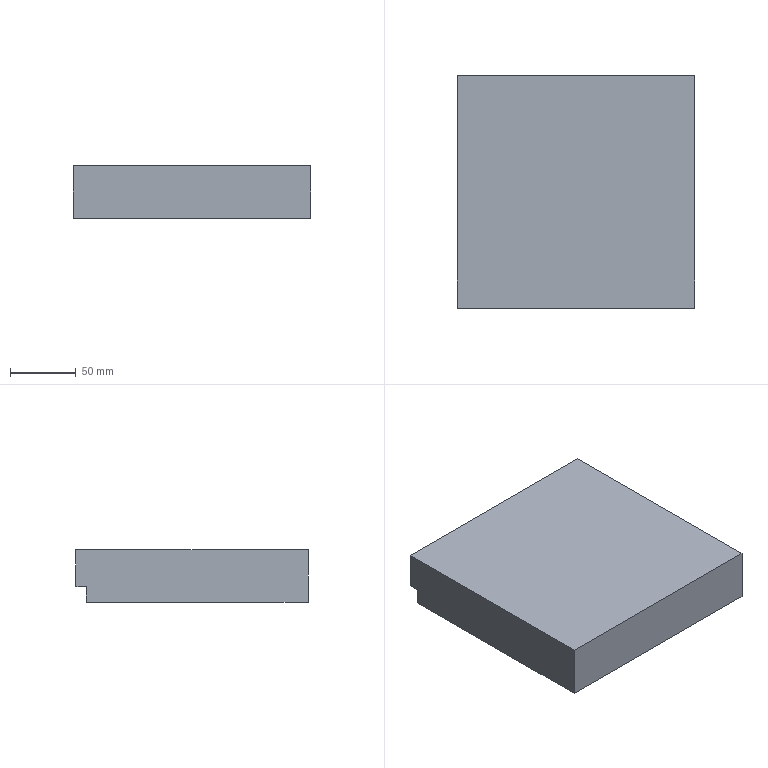Part | SolidWorks | features FlatPattern 1, ICE 1, SMBaseFlange 1, SheetMetal 1 | 1 solid | 8 faces | box 180 x 176 x 40 mm | volume 1249920 mm3 | plane 8
STEP:
#1=CARTESIAN_POINT('',(0.,168.,-28.));
#2=VERTEX_POINT('',#1);
#3=CARTESIAN_POINT('',(0.,176.,-28.));
#4=VERTEX_POINT('',#3);
#5=CARTESIAN_POINT('',(0.,168.,-28.));
#6=DIRECTION('',(0.,1.,0.));
#7=VECTOR('',#6,1000.);
#8=LINE('',#5,#7);
#9=EDGE_CURVE('',#2,#4,#8,.T.);
#10=ORIENTED_EDGE('',*,*,#9,.F.);
#11=CARTESIAN_POINT('',(0.,168.,-40.));
#12=VERTEX_POINT('',#11);
#13=CARTESIAN_POINT('',(0.,168.,-40.));
#14=DIRECTION('',(0.,0.,1.));
#15=VECTOR('',#14,1000.);
#16=LINE('',#13,#15);
#17=EDGE_CURVE('',#12,#2,#16,.T.);
#18=ORIENTED_EDGE('',*,*,#17,.F.);
#19=CARTESIAN_POINT('',(0.,0.,-40.));
#20=VERTEX_POINT('',#19);
#21=CARTESIAN_POINT('',(0.,0.,-40.));
#22=DIRECTION('',(0.,-1.,0.));
#23=VECTOR('',#22,1000.);
#24=LINE('',#21,#23);
#25=EDGE_CURVE('',#12,#20,#24,.T.);
#26=ORIENTED_EDGE('',*,*,#25,.T.);
#27=CARTESIAN_POINT('',(0.,0.,0.));
#28=VERTEX_POINT('',#27);
#29=CARTESIAN_POINT('',(0.,0.,-40.));
#30=DIRECTION('',(0.,0.,1.));
#31=VECTOR('',#30,1000.);
#32=LINE('',#29,#31);
#33=EDGE_CURVE('',#20,#28,#32,.T.);
#34=ORIENTED_EDGE('',*,*,#33,.T.);
#35=CARTESIAN_POINT('',(0.,176.,0.));
#36=VERTEX_POINT('',#35);
#37=CARTESIAN_POINT('',(0.,0.,0.));
#38=DIRECTION('',(0.,-1.,0.));
#39=VECTOR('',#38,1000.);
#40=LINE('',#37,#39);
#41=EDGE_CURVE('',#36,#28,#40,.T.);
#42=ORIENTED_EDGE('',*,*,#41,.F.);
#43=CARTESIAN_POINT('',(0.,176.,-40.));
#44=DIRECTION('',(0.,0.,1.));
#45=VECTOR('',#44,1000.);
#46=LINE('',#43,#45);
#47=EDGE_CURVE('',#4,#36,#46,.T.);
#48=ORIENTED_EDGE('',*,*,#47,.F.);
#49=EDGE_LOOP('',(#10,#18,#26,#34,#42,#48));
#50=FACE_OUTER_BOUND('',#49,.T.);
#51=CARTESIAN_POINT('',(0.,0.,-40.));
#52=DIRECTION('',(-1.,0.,0.));
#53=DIRECTION('',(0.,0.,1.));
#54=AXIS2_PLACEMENT_3D('',#51,#52,#53);
#55=PLANE('',#54);
#56=ADVANCED_FACE('',(#50),#55,.T.);
#57=CARTESIAN_POINT('',(180.,176.,-28.));
#58=VERTEX_POINT('',#57);
#59=CARTESIAN_POINT('',(180.,176.,-28.));
#60=DIRECTION('',(-1.,0.,0.));
#61=VECTOR('',#60,1000.);
#62=LINE('',#59,#61);
#63=EDGE_CURVE('',#58,#4,#62,.T.);
#64=ORIENTED_EDGE('',*,*,#63,.T.);
#65=ORIENTED_EDGE('',*,*,#47,.T.);
#66=CARTESIAN_POINT('',(180.,176.,0.));
#67=VERTEX_POINT('',#66);
#68=CARTESIAN_POINT('',(0.,176.,0.));
#69=DIRECTION('',(-1.,0.,0.));
#70=VECTOR('',#69,1000.);
#71=LINE('',#68,#70);
#72=EDGE_CURVE('',#67,#36,#71,.T.);
#73=ORIENTED_EDGE('',*,*,#72,.F.);
#74=CARTESIAN_POINT('',(180.,176.,-40.));
#75=DIRECTION('',(0.,0.,1.));
#76=VECTOR('',#75,1000.);
#77=LINE('',#74,#76);
#78=EDGE_CURVE('',#58,#67,#77,.T.);
#79=ORIENTED_EDGE('',*,*,#78,.F.);
#80=EDGE_LOOP('',(#64,#65,#73,#79));
#81=FACE_OUTER_BOUND('',#80,.T.);
#82=CARTESIAN_POINT('',(0.,176.,-40.));
#83=DIRECTION('',(0.,1.,0.));
#84=DIRECTION('',(0.,0.,1.));
#85=AXIS2_PLACEMENT_3D('',#82,#83,#84);
#86=PLANE('',#85);
#87=ADVANCED_FACE('',(#81),#86,.T.);
#88=CARTESIAN_POINT('',(180.,168.,-28.));
#89=VERTEX_POINT('',#88);
#90=CARTESIAN_POINT('',(180.,168.,-28.));
#91=DIRECTION('',(0.,1.,0.));
#92=VECTOR('',#91,1000.);
#93=LINE('',#90,#92);
#94=EDGE_CURVE('',#89,#58,#93,.T.);
#95=ORIENTED_EDGE('',*,*,#94,.T.);
#96=ORIENTED_EDGE('',*,*,#78,.T.);
#97=CARTESIAN_POINT('',(180.,0.,0.));
#98=VERTEX_POINT('',#97);
#99=CARTESIAN_POINT('',(180.,0.,0.));
#100=DIRECTION('',(0.,1.,0.));
#101=VECTOR('',#100,1000.);
#102=LINE('',#99,#101);
#103=EDGE_CURVE('',#98,#67,#102,.T.);
#104=ORIENTED_EDGE('',*,*,#103,.F.);
#105=CARTESIAN_POINT('',(180.,0.,-40.));
#106=VERTEX_POINT('',#105);
#107=CARTESIAN_POINT('',(180.,0.,-40.));
#108=DIRECTION('',(0.,0.,1.));
#109=VECTOR('',#108,1000.);
#110=LINE('',#107,#109);
#111=EDGE_CURVE('',#106,#98,#110,.T.);
#112=ORIENTED_EDGE('',*,*,#111,.F.);
#113=CARTESIAN_POINT('',(180.,168.,-40.));
#114=VERTEX_POINT('',#113);
#115=CARTESIAN_POINT('',(180.,0.,-40.));
#116=DIRECTION('',(0.,1.,0.));
#117=VECTOR('',#116,1000.);
#118=LINE('',#115,#117);
#119=EDGE_CURVE('',#106,#114,#118,.T.);
#120=ORIENTED_EDGE('',*,*,#119,.T.);
#121=CARTESIAN_POINT('',(180.,168.,-40.));
#122=DIRECTION('',(0.,0.,1.));
#123=VECTOR('',#122,1000.);
#124=LINE('',#121,#123);
#125=EDGE_CURVE('',#114,#89,#124,.T.);
#126=ORIENTED_EDGE('',*,*,#125,.T.);
#127=EDGE_LOOP('',(#95,#96,#104,#112,#120,#126));
#128=FACE_OUTER_BOUND('',#127,.T.);
#129=CARTESIAN_POINT('',(180.,0.,-40.));
#130=DIRECTION('',(1.,0.,0.));
#131=DIRECTION('',(0.,0.,-1.));
#132=AXIS2_PLACEMENT_3D('',#129,#130,#131);
#133=PLANE('',#132);
#134=ADVANCED_FACE('',(#128),#133,.T.);
#135=CARTESIAN_POINT('',(0.,0.,0.));
#136=DIRECTION('',(1.,0.,0.));
#137=VECTOR('',#136,1000.);
#138=LINE('',#135,#137);
#139=EDGE_CURVE('',#28,#98,#138,.T.);
#140=ORIENTED_EDGE('',*,*,#139,.F.);
#141=ORIENTED_EDGE('',*,*,#33,.F.);
#142=CARTESIAN_POINT('',(0.,0.,-40.));
#143=DIRECTION('',(1.,0.,0.));
#144=VECTOR('',#143,1000.);
#145=LINE('',#142,#144);
#146=EDGE_CURVE('',#20,#106,#145,.T.);
#147=ORIENTED_EDGE('',*,*,#146,.T.);
#148=ORIENTED_EDGE('',*,*,#111,.T.);
#149=EDGE_LOOP('',(#140,#141,#147,#148));
#150=FACE_OUTER_BOUND('',#149,.T.);
#151=CARTESIAN_POINT('',(0.,0.,-40.));
#152=DIRECTION('',(0.,-1.,0.));
#153=DIRECTION('',(0.,0.,-1.));
#154=AXIS2_PLACEMENT_3D('',#151,#152,#153);
#155=PLANE('',#154);
#156=ADVANCED_FACE('',(#150),#155,.T.);
#157=CARTESIAN_POINT('',(180.,168.,-40.));
#158=DIRECTION('',(-1.,0.,0.));
#159=VECTOR('',#158,1000.);
#160=LINE('',#157,#159);
#161=EDGE_CURVE('',#114,#12,#160,.T.);
#162=ORIENTED_EDGE('',*,*,#161,.F.);
#163=ORIENTED_EDGE('',*,*,#119,.F.);
#164=ORIENTED_EDGE('',*,*,#146,.F.);
#165=ORIENTED_EDGE('',*,*,#25,.F.);
#166=EDGE_LOOP('',(#162,#163,#164,#165));
#167=FACE_OUTER_BOUND('',#166,.T.);
#168=CARTESIAN_POINT('',(0.,176.,-40.));
#169=DIRECTION('',(0.,0.,-1.));
#170=DIRECTION('',(-1.,0.,0.));
#171=AXIS2_PLACEMENT_3D('',#168,#169,#170);
#172=PLANE('',#171);
#173=ADVANCED_FACE('',(#167),#172,.T.);
#174=ORIENTED_EDGE('',*,*,#41,.T.);
#175=ORIENTED_EDGE('',*,*,#139,.T.);
#176=ORIENTED_EDGE('',*,*,#103,.T.);
#177=ORIENTED_EDGE('',*,*,#72,.T.);
#178=EDGE_LOOP('',(#174,#175,#176,#177));
#179=FACE_OUTER_BOUND('',#178,.T.);
#180=CARTESIAN_POINT('',(0.,176.,0.));
#181=DIRECTION('',(0.,0.,-1.));
#182=DIRECTION('',(-1.,0.,0.));
#183=AXIS2_PLACEMENT_3D('',#180,#181,#182);
#184=PLANE('',#183);
#185=ADVANCED_FACE('',(#179),#184,.F.);
#186=ORIENTED_EDGE('',*,*,#9,.T.);
#187=ORIENTED_EDGE('',*,*,#63,.F.);
#188=ORIENTED_EDGE('',*,*,#94,.F.);
#189=CARTESIAN_POINT('',(180.,168.,-28.));
#190=DIRECTION('',(-1.,0.,0.));
#191=VECTOR('',#190,1000.);
#192=LINE('',#189,#191);
#193=EDGE_CURVE('',#89,#2,#192,.T.);
#194=ORIENTED_EDGE('',*,*,#193,.T.);
#195=EDGE_LOOP('',(#186,#187,#188,#194));
#196=FACE_OUTER_BOUND('',#195,.T.);
#197=CARTESIAN_POINT('',(180.,168.,-28.));
#198=DIRECTION('',(0.,0.,1.));
#199=DIRECTION('',(1.,0.,0.));
#200=AXIS2_PLACEMENT_3D('',#197,#198,#199);
#201=PLANE('',#200);
#202=ADVANCED_FACE('',(#196),#201,.F.);
#203=ORIENTED_EDGE('',*,*,#17,.T.);
#204=ORIENTED_EDGE('',*,*,#193,.F.);
#205=ORIENTED_EDGE('',*,*,#125,.F.);
#206=ORIENTED_EDGE('',*,*,#161,.T.);
#207=EDGE_LOOP('',(#203,#204,#205,#206));
#208=FACE_OUTER_BOUND('',#207,.T.);
#209=CARTESIAN_POINT('',(180.,168.,-40.));
#210=DIRECTION('',(0.,-1.,0.));
#211=DIRECTION('',(0.,0.,-1.));
#212=AXIS2_PLACEMENT_3D('',#209,#210,#211);
#213=PLANE('',#212);
#214=ADVANCED_FACE('',(#208),#213,.F.);
#215=CLOSED_SHELL('',(#56,#87,#134,#156,#173,#185,#202,#214));
#216=MANIFOLD_SOLID_BREP('',#215);
#217=CARTESIAN_POINT('',(0.,0.,0.));
#218=DIRECTION('',(0.,0.,1.));
#219=DIRECTION('',(1.,0.,0.));
#220=AXIS2_PLACEMENT_3D('',#217,#218,#219);
#221=(LENGTH_UNIT()NAMED_UNIT(*)SI_UNIT(.MILLI.,.METRE.));
#222=UNCERTAINTY_MEASURE_WITH_UNIT(LENGTH_MEASURE(0.00001),#221,'','');
#223=(NAMED_UNIT(*)PLANE_ANGLE_UNIT()SI_UNIT($,.RADIAN.));
#224=(NAMED_UNIT(*)SI_UNIT($,.STERADIAN.)SOLID_ANGLE_UNIT());
#225=(GEOMETRIC_REPRESENTATION_CONTEXT(3)GLOBAL_UNCERTAINTY_ASSIGNED_CONTEXT((#222))GLOBAL_UNIT_ASSIGNED_CONTEXT((#221,#223,#224))REPRESENTATION_CONTEXT('',''));
#226=ADVANCED_BREP_SHAPE_REPRESENTATION('',(#216,#220),#225);